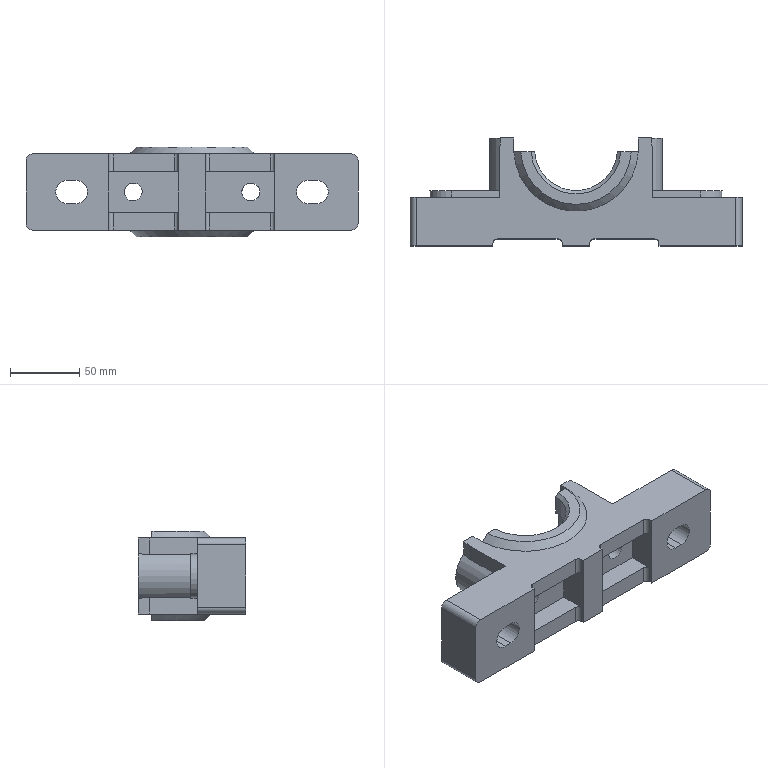Part | NX | features DATUM_CSYS 7, EXTRUDE 6, SKETCH 6, CYLINDER 3, SIMPLE HOLE 3, ABSOLUTE_DATUM_PLANE 2, CHAMFER 2, HOLE PACKAGE 2, BLEND 1 | 1 solid | 82 faces | box 240 x 78 x 65 mm | volume 522109 mm3 | plane 49 | cylinder 29 | cone 4 | commonest cylinder face diameters 6 x8 10 x4 17 x4 110 x4 13 x2 32 x2